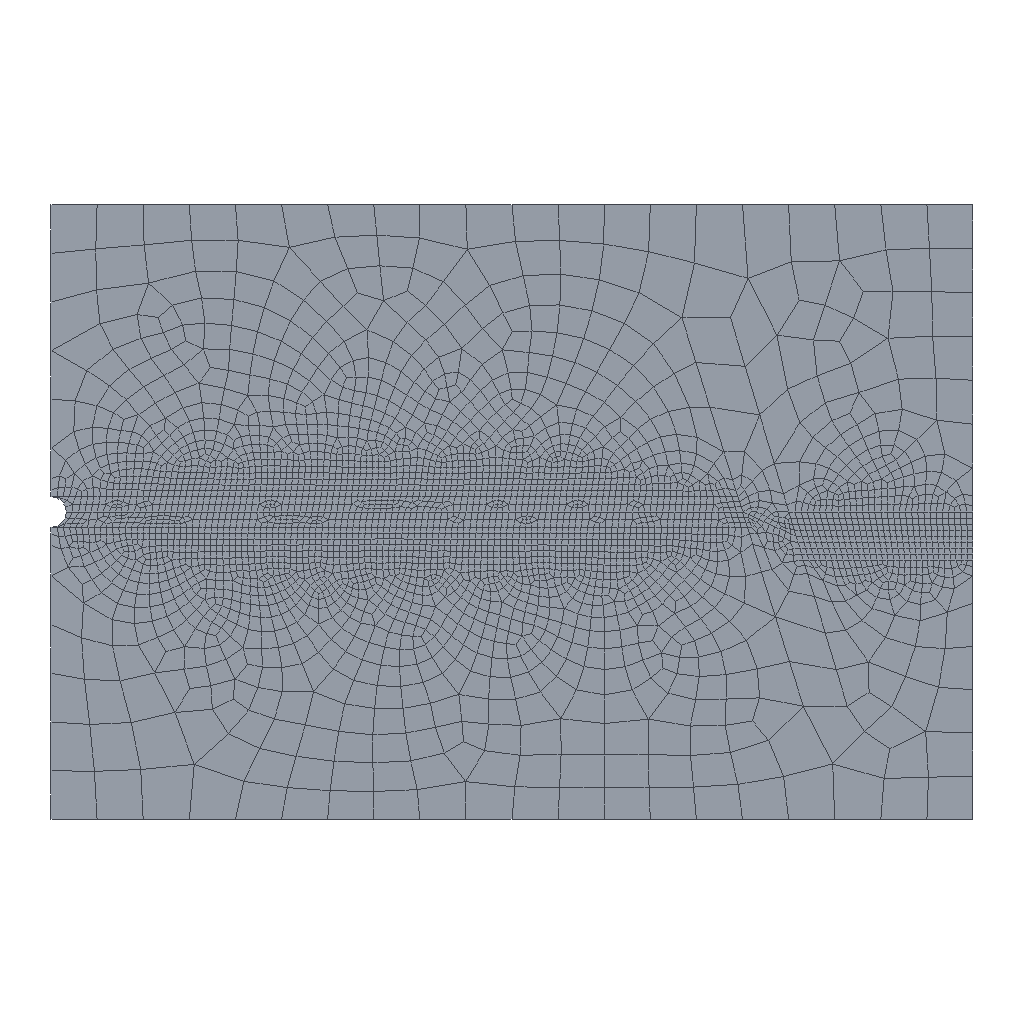Simulation study | abaqus
Set-up summary:
category,name,step,type,value,unit,region
solver,abaqus
solver,version,,,Abaqus/Standard 2020
units,not stated in the deck,,not stated
analysis,deck,,geostatic,geostatic
load_step,geo,geo,geostatic
load_step,Step-1,Step-1,soils
load_step,requested,,,2
mesh,nodes,,,4023
mesh,elements,,,3825
element_type,CPE4RP,,plane,3675
element_type,COH2D4P,,cohesive,150
load,load commands in deck,,count,1
bc,support commands in deck,,count,3
material,COH,,in results
material,COH-COPY,,in results
material,CUXINGQU,,in results
material,ROCK,,in results
check,setup vs results,,match,"per instance, exact: element labels, types and connectivity; labels of the nodes the elements use; coordinates of those nodes at SINGLE_PRECISION in 1 of 1 instance(s)"
Abaqus input file, long lists of numbers shortened:
*Heading
** Job name: Job-1 Model name: Model-1
** Generated by: Abaqus/CAE 2020
*Preprint, echo=NO, model=NO, history=NO, contact=NO
**
** PARTS
**
*Part, name=work
*Node
      1,          30.,         -10.
      2,   24.01,         -10.
** (4021 more lines like these left out)
*Element, type=CPE4RP
  1,    1,   21,  559,   84
  2,   21,   22,  560,  559
** (3673 more lines like these left out)
*Element, type=COH2D4P
3676, 3722, 3871,    9,  235, 3874, 3873
3677, 3723, 3722,  235,  236, 3875, 3874
** (148 more lines like these left out)
*Nset, nset=Set-121
    1,    2,    7,    8,    9,   10,   11,   12,   13,   14,   15,   16,   21,   22,   23,   24
   25,   26,   27,   28,   29,   30,   31,   32,   33,   34,   35,   36,   37,   38,   39,   40
** (136 more lines like these left out)
*Elset, elset=Set-121
    1,    2,    3,    4,    5,    6,    7,    8,    9,   10,   11,   12,   13,   14,   15,   16
   17,   18,   19,   20,   21,   22,   23,   24,   25,   26,   27,   28,   29,   30,   31,   32
** (123 more lines like these left out)
*Nset, nset=Set-120
    1,    2,    3,    4,    5,    6,   21,   22,   23,   24,   25,   26,   27,   28,   29,   30
   31,   32,   33,   34,   35,   36,   37,   38,   39,   40,   41,   42,   43,   44,   45,   46
** (18 more lines like these left out)
*Elset, elset=Set-120, generate
   1,  240,    1
*Nset, nset=Set-122
    1,    2,    3,    5,    6,    7,    8,    9,   10,   11,   12,   13,   14,   15,   16,   17
   18,   19,   20,   21,   22,   23,   24,   25,   26,   27,   28,   29,   30,   31,   32,   33
** (225 more lines like these left out)
*Elset, elset=Set-122, generate
  241,  3675,     1
*Elset, elset=CohesiveSeam-1-Elements, generate
 3676,  3825,     1
*Nset, nset=CohesiveSeam-1-TopNodes
   3,   4,   9,  10,  53,  54,  55,  56,  57,  58,  59,  60,  61,  62,  63,  64
  65,  66,  67,  68,  69,  70,  71,  72,  73,  74,  75,  76,  77,  78,  79,  80
** (8 more lines like these left out)
*Nset, nset=CohesiveSeam-1-BottomNodes, generate
 3722,  3872,     1
*Nset, nset=CohesiveSeam-1-MidNodes, generate
 3873,  4023,     1
*Nset, nset=inject
 3873,
*Elset, elset=initialcrack, generate
 3676,  3687,     1
*Elset, elset=__PickedSurf224_S2, internal
 1823, 1831, 1834, 1845, 1846, 1865, 1868, 1870, 1880, 1894, 1895, 1903, 1912, 1917, 1934, 1935
 1960, 1971, 1973, 1988, 1992, 1994, 1995, 2007, 2044, 2053, 2054, 2056
*Elset, elset=__PickedSurf224_S4, internal
 1825, 1847, 1849, 1854, 1861, 1866, 1890, 1892, 1900, 1901, 1906, 1909, 1913, 1914, 1915, 1919
 1922, 1929, 1936, 1937, 1940, 1950, 1956, 1957, 1959, 1979, 1984, 1986, 1989, 1990, 1991, 1996
** (1 more lines like these left out)
*Elset, elset=__PickedSurf224_S3, internal
 1828, 1830, 1833, 1838, 1843, 1844, 1856, 1863, 1864, 1867, 1891, 1905, 1908, 1928, 1931, 1933
 1948, 1975, 1997, 1998, 1999, 2003, 2009, 2010, 2038, 2052, 2060, 2068, 2069, 2070, 2071, 2072
** (3 more lines like these left out)
*Elset, elset=__PickedSurf224_S1, internal
 1842, 1869, 1871, 1896, 1918, 1980, 1987, 2004
*Surface, type=ELEMENT, name=_PickedSurf224, internal
__PickedSurf224_S2, S2
__PickedSurf224_S4, S4
__PickedSurf224_S3, S3
__PickedSurf224_S1, S1
*Elset, elset=__PickedSurf238_S2, internal
 1823, 1831, 1834, 1845, 1846, 1865, 1868, 1870, 1880, 1894, 1895, 1903, 1912, 1917, 1934, 1935
 1960, 1971, 1973, 1988, 1992, 1994, 1995, 2007, 2044, 2053, 2054, 2056
*Elset, elset=__PickedSurf238_S4, internal
 1825, 1847, 1849, 1854, 1861, 1866, 1890, 1892, 1900, 1901, 1906, 1909, 1913, 1914, 1915, 1919
 1922, 1929, 1936, 1937, 1940, 1950, 1956, 1957, 1959, 1979, 1984, 1986, 1989, 1990, 1991, 1996
** (1 more lines like these left out)
*Elset, elset=__PickedSurf238_S3, internal
 1828, 1830, 1833, 1838, 1843, 1844, 1856, 1863, 1864, 1867, 1891, 1905, 1908, 1928, 1931, 1933
 1948, 1975, 1997, 1998, 1999, 2003, 2009, 2010, 2038, 2052, 2060, 2068, 2069, 2070, 2071, 2072
** (3 more lines like these left out)
*Elset, elset=__PickedSurf238_S1, internal
 1842, 1869, 1871, 1896, 1918, 1980, 1987, 2004
*Surface, type=ELEMENT, name=_PickedSurf238, internal
__PickedSurf238_S2, S2
__PickedSurf238_S4, S4
__PickedSurf238_S3, S3
__PickedSurf238_S1, S1
*Elset, elset=_CohesiveSeam-1-TopSurf_S3, internal, generate
 3676,  3825,     1
*Surface, type=ELEMENT, name=CohesiveSeam-1-TopSurf
_CohesiveSeam-1-TopSurf_S3, S3
*Elset, elset=_CohesiveSeam-1-BottomSurf_S1, internal, generate
 3676,  3825,     1
*Surface, type=ELEMENT, name=CohesiveSeam-1-BottomSurf
_CohesiveSeam-1-BottomSurf_S1, S1
** Section: high-cui
*Solid Section, elset=Set-120, material=cuxingqu
,
** Section: rock
*Solid Section, elset=Set-122, material=rock
,
** Section: coh
*Cohesive Section, elset=CohesiveSeam-1-Elements, controls=EC-1, material=coh-Copy, response=TRACTION SEPARATION, thickness=SPECIFIED
1.,
*End Part
**
**
** ASSEMBLY
**
*Assembly, name=Assembly
**
*Instance, name=work-1, part=work
*End Instance
**
*Nset, nset=Set-4, instance=work-1
 12, 19
*Nset, nset=Set-9, instance=work-1
 12, 19
*Nset, nset=Set-11, instance=work-1
 12, 19
*Nset, nset=Set-12, instance=work-1
 12, 19
*Nset, nset=Set-19, instance=work-1
 12, 19
*Nset, nset=Set-21, instance=work-1
 12, 19
*Nset, nset=Set-29, instance=work-1
 12, 19
*Nset, nset=Set-30, instance=work-1
   8,  12,  15,  19, 373, 374, 375, 376, 377, 378, 379, 526, 527, 528, 529, 530
 531, 532
*Elset, elset=Set-30, instance=work-1
  565,  596,  597,  599,  661,  663, 1405, 1787, 2193, 2195, 2196, 2289, 2290, 2386, 2740, 3049
*Nset, nset=Set-31, instance=work-1
   8,  12,  15,  19, 373, 374, 375, 376, 377, 378, 379, 526, 527, 528, 529, 530
 531, 532
*Elset, elset=Set-31, instance=work-1
  565,  596,  597,  599,  661,  663, 1405, 1787, 2193, 2195, 2196, 2289, 2290, 2386, 2740, 3049
*Nset, nset=Set-32, instance=work-1
    1,    2,    7,    8,   11,   12,   13,   14,   15,   19,   21,   22,   23,   24,   25,   26
   27,   28,   29,   30,   31,   32,   33,   34,   35,   36,   37,   38,   39,   40,   41,   42
** (104 more lines like these left out)
*Elset, elset=Set-32, instance=work-1
  241,  242,  243,  244,  245,  246,  247,  248,  249,  250,  251,  252,  253,  254,  255,  256
  257,  258,  259,  260,  261,  262,  263,  264,  265,  266,  267,  268,  269,  270,  271,  272
** (98 more lines like these left out)
*Nset, nset=Set-35, instance=work-1
    1,    2,    7,    8,   11,   12,   13,   14,   21,   22,   23,   24,   25,   26,   27,   28
   29,   30,   31,   32,   33,   34,   35,   36,   37,   38,   39,   40,   41,   42,   43,   44
** (103 more lines like these left out)
*Elset, elset=Set-35, instance=work-1, generate
  241,  1819,     1
*Nset, nset=Set-36, instance=work-1
    1,    8,   11,   12,   15,   19,  231,  232,  233,  234,  346,  347,  348,  349,  350,  351
  352,  353,  373,  374,  375,  376,  377,  378,  379,  526,  527,  528,  529,  530,  531,  532
** (1 more lines like these left out)
*Elset, elset=Set-36, instance=work-1
  365,  366,  402,  425,  457,  542,  543,  545,  565,  596,  597,  599,  614,  654,  661,  663
  874,  876,  880, 1405, 1766, 1787, 2193, 2195, 2196, 2289, 2290, 2386, 2740, 3049
*Nset, nset=Set-37, instance=work-1
    1,    8,   11,   12,   15,   19,  231,  232,  233,  234,  346,  347,  348,  349,  350,  351
  352,  353,  373,  374,  375,  376,  377,  378,  379,  526,  527,  528,  529,  530,  531,  532
** (1 more lines like these left out)
*Elset, elset=Set-37, instance=work-1
  365,  366,  402,  425,  457,  542,  543,  545,  565,  596,  597,  599,  614,  654,  661,  663
  874,  876,  880, 1405, 1766, 1787, 2193, 2195, 2196, 2289, 2290, 2386, 2740, 3049
*Nset, nset=Set-38, instance=work-1
    1,    2,    7,    8,   11,   12,   13,   14,   15,   19,   21,   22,   23,   24,   25,   26
   27,   28,   29,   30,   31,   32,   33,   34,   35,   36,   37,   38,   39,   40,   41,   42
** (104 more lines like these left out)
*Elset, elset=Set-38, instance=work-1
  241,  242,  243,  244,  245,  246,  247,  248,  249,  250,  251,  252,  253,  254,  255,  256
  257,  258,  259,  260,  261,  262,  263,  264,  265,  266,  267,  268,  269,  270,  271,  272
** (98 more lines like these left out)
*Nset, nset=Set-39, instance=work-1
    1,    8,   11,   12,   15,   19,  231,  232,  233,  234,  346,  347,  348,  349,  350,  351
  352,  353,  373,  374,  375,  376,  377,  378,  379,  526,  527,  528,  529,  530,  531,  532
** (1 more lines like these left out)
*Elset, elset=Set-39, instance=work-1
  365,  366,  402,  425,  457,  542,  543,  545,  565,  596,  597,  599,  614,  654,  661,  663
  874,  876,  880, 1405, 1766, 1787, 2193, 2195, 2196, 2289, 2290, 2386, 2740, 3049
*Nset, nset=Set-40, instance=work-1
   8,  12,  15,  19, 373, 374, 375, 376, 377, 378, 379, 526, 527, 528, 529, 530
 531, 532
*Elset, elset=Set-40, instance=work-1
  565,  596,  597,  599,  661,  663, 1405, 1787, 2193, 2195, 2196, 2289, 2290, 2386, 2740, 3049
*Nset, nset=Set-41, instance=work-1
    1,    2,    7,    8,    9,   10,   11,   12,   13,   14,   15,   16,   19,   21,   22,   23
   24,   25,   26,   27,   28,   29,   30,   31,   32,   33,   34,   35,   36,   37,   38,   39
** (137 more lines like these left out)
*Elset, elset=Set-41, instance=work-1
    1,    2,    3,    4,    5,    6,    7,    8,    9,   10,   11,   12,   13,   14,   15,   16
   17,   18,   19,   20,   21,   22,   23,   24,   25,   26,   27,   28,   29,   30,   31,   32
** (124 more lines like these left out)
*Nset, nset=Set-42, instance=work-1
    1,    2,    8,   11,   50,   51,   52,  231,  232,  233,  234,  346,  347,  348,  349,  350
  351,  352,  353, 3841, 3871
*Elset, elset=Set-42, instance=work-1
   30,   60,   90,  120,  365,  366,  402,  425,  457,  542,  543,  545,  614,  654,  874,  876
  880, 1766, 2127, 2128, 2149, 2153
*Nset, nset=Set-43, instance=work-1
    1,    2,    7,    8,    9,   10,   11,   12,   13,   14,   15,   16,   21,   22,   23,   24
   25,   26,   27,   28,   29,   30,   31,   32,   33,   34,   35,   36,   37,   38,   39,   40
** (136 more lines like these left out)
*Elset, elset=Set-43, instance=work-1
    1,    2,    3,    4,    5,    6,    7,    8,    9,   10,   11,   12,   13,   14,   15,   16
   17,   18,   19,   20,   21,   22,   23,   24,   25,   26,   27,   28,   29,   30,   31,   32
** (123 more lines like these left out)
*Nset, nset=Set-44, instance=work-1
   7,  13, 380, 381, 382, 383, 384
*Elset, elset=Set-44, instance=work-1
  608,  745,  748,  779, 1000, 1736, 2112, 2115, 2116, 2118, 2141, 2154
*Nset, nset=Set-45, instance=work-1
   8,  12,  15,  19, 373, 374, 375, 376, 377, 378, 379, 526, 527, 528, 529, 530
 531, 532
*Elset, elset=Set-45, instance=work-1
  565,  596,  597,  599,  661,  663, 1405, 1787, 2193, 2195, 2196, 2289, 2290, 2386, 2740, 3049
*Nset, nset=Set-46, instance=work-1
  11,  12,  19,  20, 354, 355, 356, 357, 358, 359, 360, 361, 362, 363, 364, 365
 366, 367, 368, 369, 370, 371, 372, 533, 534, 535, 536, 537, 538, 539, 540, 541
** (1 more lines like these left out)
*Elset, elset=Set-46, instance=work-1
  525,  526,  545,  546,  547,  553,  555,  556,  567,  568,  578,  585,  590,  596,  657,  658
  659,  660, 1761, 1772, 2160, 2161, 2162, 2178, 2179, 2180, 2190, 2191, 2196, 2197, 2198, 2199
** (1 more lines like these left out)
*Nset, nset=Set-47, instance=work-1
    1,    4,    6,   11,   20,   82,   83,   84,  114,  115,  116,  346,  347,  348,  349,  350
  351,  352,  353,  552,  553,  554,  555,  556,  557,  558, 3872
*Elset, elset=Set-47, instance=work-1
    1,   31,   61,   91,  150,  180,  210,  240,  542,  543,  545,  614,  654,  874,  876,  880
 1766, 2162, 2163, 2166, 2229, 2283, 2390, 2392, 3133
*Nset, nset=Set-48, instance=work-1, generate
    1,  3872,     1
*Elset, elset=Set-48, instance=work-1, generate
    1,  3825,     1
*Nset, nset=Set-49, instance=work-1, generate
    1,  3872,     1
*Elset, elset=Set-49, instance=work-1, generate
    1,  3675,     1
*Elset, elset=_Surf-15_S1, internal, instance=work-1
  608,  779, 1736
*Elset, elset=_Surf-15_S4, internal, instance=work-1
 745,
*Elset, elset=_Surf-15_S2, internal, instance=work-1
  748, 1000
*Surface, type=ELEMENT, name=Surf-15
_Surf-15_S1, S1
_Surf-15_S4, S4
_Surf-15_S2, S2
*Elset, elset=_Surf-16_S2, internal, instance=work-1
  30,  60,  90, 120, 365, 366, 402, 876, 880
*Elset, elset=_Surf-16_S3, internal, instance=work-1
 425, 457, 542, 543, 874
*Elset, elset=_Surf-16_S1, internal, instance=work-1
  545,  614, 1766
*Elset, elset=_Surf-16_S4, internal, instance=work-1
 654,
*Surface, type=ELEMENT, name=Surf-16
_Surf-16_S2, S2
_Surf-16_S3, S3
_Surf-16_S4, S4
_Surf-16_S1, S1
*End Assembly
**
** ELEMENT CONTROLS
**
*Section Controls, name=EC-1, ELEMENT DELETION=YES
1., 1., 1.
*Amplitude, name=Amp-1
             0.,              0.,            300.,              1.
**
** MATERIALS
**
*Material, name=coh
*Damage Initiation, criterion=MAXS
10000.,10000.,10000.
*Damage Evolution, type=DISPLACEMENT
 1e-09,
*Damage Stabilization
0.001
*Elastic, type=TRACTION
 1.5e+10, 1.5e+10, 1.5e+10
*Fluid Leakoff
 1e-14, 1e-14
*Gap Flow
 0.001,
*Material, name=coh-Copy
*Damage Initiation, criterion=MAXE
 0.0001, 0.0001, 0.0001
*Damage Evolution, type=DISPLACEMENT
 1e-19,
*Elastic, type=TRACTION
 1.5e+10, 1.5e+10, 1.5e+10
*Fluid Leakoff
 1e-14, 1e-14
*Gap Flow
 0.001,
*Material, name=cuxingqu
*Elastic
 2.92e+10, 0.278
*Permeability, specific=9800.
 5e-07, 0.25
*Material, name=rock
*Elastic
 2.65e+10, 0.29
*Permeability, specific=9800.
 5e-07, 0.25
**
** INTERACTION PROPERTIES
**
*Surface Interaction, name=IntProp-1
1.,
**
** BOUNDARY CONDITIONS
**
** Name: BC-1 Type: 对称/反对称/完全固定
*Boundary
Set-40, XSYMM
** Name: BC-2 Type: 位移/转角
*Boundary
Set-46, 2, 2
** Name: BC-3 Type: 位移/转角
*Boundary
Set-47, 1, 1
**
** PREDEFINED FIELDS
**
** Name: Predefined Field-1   Type: Void ratio
*Initial Conditions, TYPE=RATIO
Set-48, 0.2
** Name: Predefined Field-2   Type: Stress
*Initial Conditions, type=STRESS
Set-49, -10000., -10000., -10000., 0.,
** ----------------------------------------------------------------
*initial conditions,type=initial gap
work-1.initialcrack
**
** STEP: geo
**
*Step, name=geo, nlgeom=NO, unsymm=YES
*Geostatic
**
** CONTROLS
**
*Controls, reset
*Controls, parameters=time incrementation
, , , , , , , 20, , ,
**
** OUTPUT REQUESTS
**
*Restart, write, frequency=0
**
** FIELD OUTPUT: F-Output-1
**
*Output, field
*Node Output
CF, PHILSM, POR, PSILSM, RF, U
*Element Output, directions=YES
E, FLUVR, FLVEL, LE, LOADSXFEM, MISES, PFOPENXFEM, S, SAT, SDEG
*Contact Output
CSDMG, PFL, PFLA, PTL, PTLA
*Output, history, frequency=0
*End Step
** ----------------------------------------------------------------
**
** STEP: Step-1
**
*Step, name=Step-1, nlgeom=YES, inc=10000, unsymm=YES
*Soils, consolidation, end=PERIOD, utol=1e+19, creep=none
0.01, 50., 3e-06, 50.,
**
** LOADS
**
** Name: Load-3   Type: Concentrated pore fluid
*Cflow, amplitude=Amp-1
work-1.inject,  , -0.005
**
** CONTROLS
**
*Controls, reset
*Controls, parameters=time incrementation
, , , , , , , 20, , ,
**
** OUTPUT REQUESTS
**
*Restart, write, frequency=0
**
** FIELD OUTPUT: F-Output-1
**
*Output, field
*Node Output
CF, PHILSM, POR, PSILSM, RF, U
*Element Output, directions=YES
E, FLUVR, FLVEL, LE, MISES, S, SAT, SDEG, VOIDR, pfopen
*Contact Output
CSDMG, PFL, PFLA, PTL, PTLA
**
** HISTORY OUTPUT: H-Output-1
**
*Output, history
*Node Output, nset=work-1.inject
POR,
*End Step
Results summary:
result,step,,completed,increments=1 time=1.0/1.0
result,step,,completed,increments=34 time=50.0/50.0
result,analysis,,,"soils, consolidation"
result,last_loadstep,,,2
result,primary field,,,"U, POR"
result,reaction total,,FX,-200.0,model units
result,reaction total,,FY,320.0,model units
result,reaction total,,FZ,0.0,model units